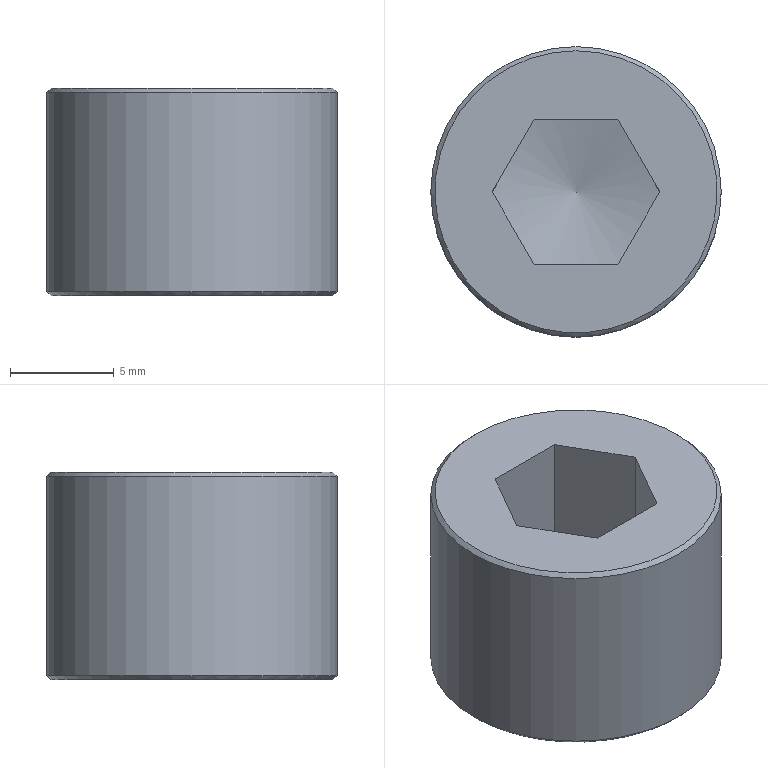Part | NX | features MFD10-WL40_3 2 | 1 solid | 18 faces | box 14 x 14 x 10 mm | volume 1223 mm3 | plane 14 | cone 3 | cylinder 1 | commonest cylinder face diameters 14 x1
STEP:
#1=CARTESIAN_POINT('',(275.029,-404.95,147.75));
#2=VERTEX_POINT('',#1);
#3=CARTESIAN_POINT('',(275.029,-411.95,147.75));
#4=DIRECTION('',(0.,0.,1.));
#5=DIRECTION('',(0.,-1.,0.));
#6=AXIS2_PLACEMENT_3D('',#3,#4,#5);
#7=CIRCLE('',#6,7.);
#8=EDGE_CURVE('',#2,#2,#7,.T.);
#9=ORIENTED_EDGE('',*,*,#8,.T.);
#10=EDGE_LOOP('',(#9));
#11=FACE_BOUND('',#10,.T.);
#12=CARTESIAN_POINT('',(275.029,-405.15,147.95));
#13=VERTEX_POINT('',#12);
#14=CARTESIAN_POINT('',(275.029,-411.95,147.95));
#15=DIRECTION('',(0.,0.,-1.));
#16=DIRECTION('',(0.,-1.,0.));
#17=AXIS2_PLACEMENT_3D('',#14,#15,#16);
#18=CIRCLE('',#17,6.8);
#19=EDGE_CURVE('',#13,#13,#18,.T.);
#20=ORIENTED_EDGE('',*,*,#19,.T.);
#21=EDGE_LOOP('',(#20));
#22=FACE_BOUND('',#21,.T.);
#23=CARTESIAN_POINT('',(275.029,-411.95,147.95));
#24=DIRECTION('',(0.,0.,-1.));
#25=DIRECTION('',(0.,-1.,0.));
#26=AXIS2_PLACEMENT_3D('',#23,#24,#25);
#27=CONICAL_SURFACE('',#26,6.8,0.7854);
#28=ADVANCED_FACE('',(#11,#22),#27,.T.);
#29=CARTESIAN_POINT('',(275.029,-404.95,138.15));
#30=VERTEX_POINT('',#29);
#31=CARTESIAN_POINT('',(275.029,-411.95,138.15));
#32=DIRECTION('',(0.,0.,-1.));
#33=DIRECTION('',(0.,-1.,0.));
#34=AXIS2_PLACEMENT_3D('',#31,#32,#33);
#35=CIRCLE('',#34,7.);
#36=EDGE_CURVE('',#30,#30,#35,.T.);
#37=ORIENTED_EDGE('',*,*,#36,.F.);
#38=EDGE_LOOP('',(#37));
#39=FACE_BOUND('',#38,.T.);
#40=ORIENTED_EDGE('',*,*,#8,.F.);
#41=EDGE_LOOP('',(#40));
#42=FACE_BOUND('',#41,.T.);
#43=CARTESIAN_POINT('',(275.029,-411.95,142.95));
#44=DIRECTION('',(0.,0.,-1.));
#45=DIRECTION('',(0.,1.,0.));
#46=AXIS2_PLACEMENT_3D('',#43,#44,#45);
#47=CYLINDRICAL_SURFACE('',#46,7.);
#48=ADVANCED_FACE('',(#39,#42),#47,.T.);
#49=CARTESIAN_POINT('',(270.987,-411.95,147.95));
#50=VERTEX_POINT('',#49);
#51=CARTESIAN_POINT('',(273.008,-408.45,147.95));
#52=VERTEX_POINT('',#51);
#53=CARTESIAN_POINT('',(271.997,-410.2,147.95));
#54=DIRECTION('',(0.5,0.866,0.));
#55=VECTOR('',#54,1000.);
#56=LINE('',#53,#55);
#57=EDGE_CURVE('',#50,#52,#56,.T.);
#58=ORIENTED_EDGE('',*,*,#57,.T.);
#59=CARTESIAN_POINT('',(277.049,-408.45,147.95));
#60=VERTEX_POINT('',#59);
#61=CARTESIAN_POINT('',(275.029,-408.45,147.95));
#62=DIRECTION('',(1.,0.,0.));
#63=VECTOR('',#62,1000.);
#64=LINE('',#61,#63);
#65=EDGE_CURVE('',#52,#60,#64,.T.);
#66=ORIENTED_EDGE('',*,*,#65,.T.);
#67=CARTESIAN_POINT('',(279.07,-411.95,147.95));
#68=VERTEX_POINT('',#67);
#69=CARTESIAN_POINT('',(278.06,-410.2,147.95));
#70=DIRECTION('',(0.5,-0.866,0.));
#71=VECTOR('',#70,1000.);
#72=LINE('',#69,#71);
#73=EDGE_CURVE('',#60,#68,#72,.T.);
#74=ORIENTED_EDGE('',*,*,#73,.T.);
#75=CARTESIAN_POINT('',(277.049,-415.45,147.95));
#76=VERTEX_POINT('',#75);
#77=CARTESIAN_POINT('',(278.06,-413.7,147.95));
#78=DIRECTION('',(-0.5,-0.866,0.));
#79=VECTOR('',#78,1000.);
#80=LINE('',#77,#79);
#81=EDGE_CURVE('',#68,#76,#80,.T.);
#82=ORIENTED_EDGE('',*,*,#81,.T.);
#83=CARTESIAN_POINT('',(273.008,-415.45,147.95));
#84=VERTEX_POINT('',#83);
#85=CARTESIAN_POINT('',(275.029,-415.45,147.95));
#86=DIRECTION('',(-1.,0.,0.));
#87=VECTOR('',#86,1000.);
#88=LINE('',#85,#87);
#89=EDGE_CURVE('',#76,#84,#88,.T.);
#90=ORIENTED_EDGE('',*,*,#89,.T.);
#91=CARTESIAN_POINT('',(271.997,-413.7,147.95));
#92=DIRECTION('',(-0.5,0.866,0.));
#93=VECTOR('',#92,1000.);
#94=LINE('',#91,#93);
#95=EDGE_CURVE('',#84,#50,#94,.T.);
#96=ORIENTED_EDGE('',*,*,#95,.T.);
#97=EDGE_LOOP('',(#58,#66,#74,#82,#90,#96));
#98=FACE_BOUND('',#97,.T.);
#99=ORIENTED_EDGE('',*,*,#19,.F.);
#100=EDGE_LOOP('',(#99));
#101=FACE_BOUND('',#100,.T.);
#102=CARTESIAN_POINT('',(275.029,-411.95,147.95));
#103=DIRECTION('',(0.,0.,1.));
#104=DIRECTION('',(0.,-1.,0.));
#105=AXIS2_PLACEMENT_3D('',#102,#103,#104);
#106=PLANE('',#105);
#107=ADVANCED_FACE('',(#98,#101),#106,.T.);
#108=ORIENTED_EDGE('',*,*,#36,.T.);
#109=EDGE_LOOP('',(#108));
#110=FACE_BOUND('',#109,.T.);
#111=CARTESIAN_POINT('',(275.029,-405.15,137.95));
#112=VERTEX_POINT('',#111);
#113=CARTESIAN_POINT('',(275.029,-411.95,137.95));
#114=DIRECTION('',(0.,0.,1.));
#115=DIRECTION('',(0.,-1.,0.));
#116=AXIS2_PLACEMENT_3D('',#113,#114,#115);
#117=CIRCLE('',#116,6.8);
#118=EDGE_CURVE('',#112,#112,#117,.T.);
#119=ORIENTED_EDGE('',*,*,#118,.T.);
#120=EDGE_LOOP('',(#119));
#121=FACE_BOUND('',#120,.T.);
#122=CARTESIAN_POINT('',(275.029,-411.95,137.95));
#123=DIRECTION('',(0.,0.,1.));
#124=DIRECTION('',(0.,-1.,0.));
#125=AXIS2_PLACEMENT_3D('',#122,#123,#124);
#126=CONICAL_SURFACE('',#125,6.8,0.7854);
#127=ADVANCED_FACE('',(#110,#121),#126,.T.);
#128=ORIENTED_EDGE('',*,*,#118,.F.);
#129=EDGE_LOOP('',(#128));
#130=FACE_BOUND('',#129,.T.);
#131=CARTESIAN_POINT('',(275.029,-411.95,137.95));
#132=DIRECTION('',(0.,0.,-1.));
#133=DIRECTION('',(0.,1.,0.));
#134=AXIS2_PLACEMENT_3D('',#131,#132,#133);
#135=PLANE('',#134);
#136=ADVANCED_FACE('',(#130),#135,.T.);
#137=CARTESIAN_POINT('',(270.987,-411.95,140.95));
#138=VERTEX_POINT('',#137);
#139=CARTESIAN_POINT('',(273.008,-408.45,140.95));
#140=VERTEX_POINT('',#139);
#141=CARTESIAN_POINT('',(271.997,-410.2,140.95));
#142=DIRECTION('',(0.5,0.866,0.));
#143=VECTOR('',#142,1000.);
#144=LINE('',#141,#143);
#145=EDGE_CURVE('',#138,#140,#144,.T.);
#146=ORIENTED_EDGE('',*,*,#145,.F.);
#147=CARTESIAN_POINT('',(275.029,-411.95,140.95));
#148=DIRECTION('',(0.,0.,1.));
#149=DIRECTION('',(0.,1.,0.));
#150=AXIS2_PLACEMENT_3D('',#147,#148,#149);
#151=CIRCLE('',#150,4.041);
#152=EDGE_CURVE('',#140,#138,#151,.T.);
#153=ORIENTED_EDGE('',*,*,#152,.F.);
#154=EDGE_LOOP('',(#146,#153));
#155=FACE_BOUND('',#154,.T.);
#156=CARTESIAN_POINT('',(275.029,-411.95,140.95));
#157=DIRECTION('',(0.,0.,1.));
#158=DIRECTION('',(0.,-1.,0.));
#159=AXIS2_PLACEMENT_3D('',#156,#157,#158);
#160=PLANE('',#159);
#161=ADVANCED_FACE('',(#155),#160,.F.);
#162=CARTESIAN_POINT('',(277.049,-408.45,140.95));
#163=VERTEX_POINT('',#162);
#164=CARTESIAN_POINT('',(275.029,-408.45,140.95));
#165=DIRECTION('',(1.,0.,0.));
#166=VECTOR('',#165,1000.);
#167=LINE('',#164,#166);
#168=EDGE_CURVE('',#140,#163,#167,.T.);
#169=ORIENTED_EDGE('',*,*,#168,.F.);
#170=CARTESIAN_POINT('',(275.029,-411.95,140.95));
#171=DIRECTION('',(0.,0.,1.));
#172=DIRECTION('',(0.,1.,0.));
#173=AXIS2_PLACEMENT_3D('',#170,#171,#172);
#174=CIRCLE('',#173,4.041);
#175=EDGE_CURVE('',#163,#140,#174,.T.);
#176=ORIENTED_EDGE('',*,*,#175,.F.);
#177=EDGE_LOOP('',(#169,#176));
#178=FACE_BOUND('',#177,.T.);
#179=CARTESIAN_POINT('',(275.029,-411.95,140.95));
#180=DIRECTION('',(0.,0.,1.));
#181=DIRECTION('',(0.,-1.,0.));
#182=AXIS2_PLACEMENT_3D('',#179,#180,#181);
#183=PLANE('',#182);
#184=ADVANCED_FACE('',(#178),#183,.F.);
#185=CARTESIAN_POINT('',(279.07,-411.95,140.95));
#186=VERTEX_POINT('',#185);
#187=CARTESIAN_POINT('',(278.06,-410.2,140.95));
#188=DIRECTION('',(0.5,-0.866,0.));
#189=VECTOR('',#188,1000.);
#190=LINE('',#187,#189);
#191=EDGE_CURVE('',#163,#186,#190,.T.);
#192=ORIENTED_EDGE('',*,*,#191,.F.);
#193=CARTESIAN_POINT('',(275.029,-411.95,140.95));
#194=DIRECTION('',(0.,0.,1.));
#195=DIRECTION('',(0.,1.,0.));
#196=AXIS2_PLACEMENT_3D('',#193,#194,#195);
#197=CIRCLE('',#196,4.041);
#198=EDGE_CURVE('',#186,#163,#197,.T.);
#199=ORIENTED_EDGE('',*,*,#198,.F.);
#200=EDGE_LOOP('',(#192,#199));
#201=FACE_BOUND('',#200,.T.);
#202=CARTESIAN_POINT('',(275.029,-411.95,140.95));
#203=DIRECTION('',(0.,0.,1.));
#204=DIRECTION('',(0.,-1.,0.));
#205=AXIS2_PLACEMENT_3D('',#202,#203,#204);
#206=PLANE('',#205);
#207=ADVANCED_FACE('',(#201),#206,.F.);
#208=CARTESIAN_POINT('',(277.049,-415.45,140.95));
#209=VERTEX_POINT('',#208);
#210=CARTESIAN_POINT('',(278.06,-413.7,140.95));
#211=DIRECTION('',(-0.5,-0.866,0.));
#212=VECTOR('',#211,1000.);
#213=LINE('',#210,#212);
#214=EDGE_CURVE('',#186,#209,#213,.T.);
#215=ORIENTED_EDGE('',*,*,#214,.F.);
#216=CARTESIAN_POINT('',(275.029,-411.95,140.95));
#217=DIRECTION('',(0.,0.,1.));
#218=DIRECTION('',(0.,1.,0.));
#219=AXIS2_PLACEMENT_3D('',#216,#217,#218);
#220=CIRCLE('',#219,4.041);
#221=EDGE_CURVE('',#209,#186,#220,.T.);
#222=ORIENTED_EDGE('',*,*,#221,.F.);
#223=EDGE_LOOP('',(#215,#222));
#224=FACE_BOUND('',#223,.T.);
#225=CARTESIAN_POINT('',(275.029,-411.95,140.95));
#226=DIRECTION('',(0.,0.,1.));
#227=DIRECTION('',(0.,-1.,0.));
#228=AXIS2_PLACEMENT_3D('',#225,#226,#227);
#229=PLANE('',#228);
#230=ADVANCED_FACE('',(#224),#229,.F.);
#231=CARTESIAN_POINT('',(273.008,-415.45,140.95));
#232=VERTEX_POINT('',#231);
#233=CARTESIAN_POINT('',(275.029,-415.45,140.95));
#234=DIRECTION('',(-1.,0.,0.));
#235=VECTOR('',#234,1000.);
#236=LINE('',#233,#235);
#237=EDGE_CURVE('',#209,#232,#236,.T.);
#238=ORIENTED_EDGE('',*,*,#237,.F.);
#239=CARTESIAN_POINT('',(275.029,-411.95,140.95));
#240=DIRECTION('',(0.,0.,1.));
#241=DIRECTION('',(0.,1.,0.));
#242=AXIS2_PLACEMENT_3D('',#239,#240,#241);
#243=CIRCLE('',#242,4.041);
#244=EDGE_CURVE('',#232,#209,#243,.T.);
#245=ORIENTED_EDGE('',*,*,#244,.F.);
#246=EDGE_LOOP('',(#238,#245));
#247=FACE_BOUND('',#246,.T.);
#248=CARTESIAN_POINT('',(275.029,-411.95,140.95));
#249=DIRECTION('',(0.,0.,1.));
#250=DIRECTION('',(0.,-1.,0.));
#251=AXIS2_PLACEMENT_3D('',#248,#249,#250);
#252=PLANE('',#251);
#253=ADVANCED_FACE('',(#247),#252,.F.);
#254=CARTESIAN_POINT('',(271.997,-413.7,140.95));
#255=DIRECTION('',(-0.5,0.866,0.));
#256=VECTOR('',#255,1000.);
#257=LINE('',#254,#256);
#258=EDGE_CURVE('',#232,#138,#257,.T.);
#259=ORIENTED_EDGE('',*,*,#258,.F.);
#260=CARTESIAN_POINT('',(275.029,-411.95,140.95));
#261=DIRECTION('',(0.,0.,1.));
#262=DIRECTION('',(0.,1.,0.));
#263=AXIS2_PLACEMENT_3D('',#260,#261,#262);
#264=CIRCLE('',#263,4.041);
#265=EDGE_CURVE('',#138,#232,#264,.T.);
#266=ORIENTED_EDGE('',*,*,#265,.F.);
#267=EDGE_LOOP('',(#259,#266));
#268=FACE_BOUND('',#267,.T.);
#269=CARTESIAN_POINT('',(275.029,-411.95,140.95));
#270=DIRECTION('',(0.,0.,1.));
#271=DIRECTION('',(0.,-1.,0.));
#272=AXIS2_PLACEMENT_3D('',#269,#270,#271);
#273=PLANE('',#272);
#274=ADVANCED_FACE('',(#268),#273,.F.);
#275=ORIENTED_EDGE('',*,*,#175,.T.);
#276=ORIENTED_EDGE('',*,*,#152,.T.);
#277=ORIENTED_EDGE('',*,*,#265,.T.);
#278=ORIENTED_EDGE('',*,*,#244,.T.);
#279=ORIENTED_EDGE('',*,*,#221,.T.);
#280=ORIENTED_EDGE('',*,*,#198,.T.);
#281=EDGE_LOOP('',(#275,#276,#277,#278,#279,#280));
#282=FACE_BOUND('',#281,.T.);
#283=CARTESIAN_POINT('',(275.029,-411.95,139.95));
#284=VERTEX_POINT('',#283);
#285=VERTEX_LOOP('',#284);
#286=FACE_BOUND('',#285,.T.);
#287=CARTESIAN_POINT('',(275.029,-411.95,140.45));
#288=DIRECTION('',(0.,0.,1.));
#289=DIRECTION('',(0.,1.,0.));
#290=AXIS2_PLACEMENT_3D('',#287,#288,#289);
#291=CONICAL_SURFACE('',#290,2.021,1.328);
#292=ADVANCED_FACE('',(#282,#286),#291,.F.);
#293=CARTESIAN_POINT('',(270.987,-411.95,144.45));
#294=DIRECTION('',(0.,0.,1.));
#295=VECTOR('',#294,1000.);
#296=LINE('',#293,#295);
#297=EDGE_CURVE('',#138,#50,#296,.T.);
#298=ORIENTED_EDGE('',*,*,#297,.F.);
#299=ORIENTED_EDGE('',*,*,#145,.T.);
#300=CARTESIAN_POINT('',(273.008,-408.45,144.45));
#301=DIRECTION('',(0.,0.,1.));
#302=VECTOR('',#301,1000.);
#303=LINE('',#300,#302);
#304=EDGE_CURVE('',#140,#52,#303,.T.);
#305=ORIENTED_EDGE('',*,*,#304,.T.);
#306=ORIENTED_EDGE('',*,*,#57,.F.);
#307=EDGE_LOOP('',(#298,#299,#305,#306));
#308=FACE_BOUND('',#307,.T.);
#309=CARTESIAN_POINT('',(271.997,-410.2,144.45));
#310=DIRECTION('',(0.866,-0.5,0.));
#311=DIRECTION('',(0.,0.,-1.));
#312=AXIS2_PLACEMENT_3D('',#309,#310,#311);
#313=PLANE('',#312);
#314=ADVANCED_FACE('',(#308),#313,.T.);
#315=CARTESIAN_POINT('',(273.008,-415.45,144.45));
#316=DIRECTION('',(0.,0.,1.));
#317=VECTOR('',#316,1000.);
#318=LINE('',#315,#317);
#319=EDGE_CURVE('',#232,#84,#318,.T.);
#320=ORIENTED_EDGE('',*,*,#319,.F.);
#321=ORIENTED_EDGE('',*,*,#258,.T.);
#322=ORIENTED_EDGE('',*,*,#297,.T.);
#323=ORIENTED_EDGE('',*,*,#95,.F.);
#324=EDGE_LOOP('',(#320,#321,#322,#323));
#325=FACE_BOUND('',#324,.T.);
#326=CARTESIAN_POINT('',(271.997,-413.7,144.45));
#327=DIRECTION('',(0.866,0.5,0.));
#328=DIRECTION('',(0.,0.,1.));
#329=AXIS2_PLACEMENT_3D('',#326,#327,#328);
#330=PLANE('',#329);
#331=ADVANCED_FACE('',(#325),#330,.T.);
#332=CARTESIAN_POINT('',(277.049,-415.45,144.45));
#333=DIRECTION('',(0.,0.,1.));
#334=VECTOR('',#333,1000.);
#335=LINE('',#332,#334);
#336=EDGE_CURVE('',#209,#76,#335,.T.);
#337=ORIENTED_EDGE('',*,*,#336,.F.);
#338=ORIENTED_EDGE('',*,*,#237,.T.);
#339=ORIENTED_EDGE('',*,*,#319,.T.);
#340=ORIENTED_EDGE('',*,*,#89,.F.);
#341=EDGE_LOOP('',(#337,#338,#339,#340));
#342=FACE_BOUND('',#341,.T.);
#343=CARTESIAN_POINT('',(275.029,-415.45,144.45));
#344=DIRECTION('',(0.,1.,0.));
#345=DIRECTION('',(0.,0.,1.));
#346=AXIS2_PLACEMENT_3D('',#343,#344,#345);
#347=PLANE('',#346);
#348=ADVANCED_FACE('',(#342),#347,.T.);
#349=CARTESIAN_POINT('',(279.07,-411.95,144.45));
#350=DIRECTION('',(0.,0.,1.));
#351=VECTOR('',#350,1000.);
#352=LINE('',#349,#351);
#353=EDGE_CURVE('',#186,#68,#352,.T.);
#354=ORIENTED_EDGE('',*,*,#353,.F.);
#355=ORIENTED_EDGE('',*,*,#214,.T.);
#356=ORIENTED_EDGE('',*,*,#336,.T.);
#357=ORIENTED_EDGE('',*,*,#81,.F.);
#358=EDGE_LOOP('',(#354,#355,#356,#357));
#359=FACE_BOUND('',#358,.T.);
#360=CARTESIAN_POINT('',(278.06,-413.7,144.45));
#361=DIRECTION('',(-0.866,0.5,0.));
#362=DIRECTION('',(0.,0.,1.));
#363=AXIS2_PLACEMENT_3D('',#360,#361,#362);
#364=PLANE('',#363);
#365=ADVANCED_FACE('',(#359),#364,.T.);
#366=CARTESIAN_POINT('',(277.049,-408.45,144.45));
#367=DIRECTION('',(0.,0.,1.));
#368=VECTOR('',#367,1000.);
#369=LINE('',#366,#368);
#370=EDGE_CURVE('',#163,#60,#369,.T.);
#371=ORIENTED_EDGE('',*,*,#370,.F.);
#372=ORIENTED_EDGE('',*,*,#191,.T.);
#373=ORIENTED_EDGE('',*,*,#353,.T.);
#374=ORIENTED_EDGE('',*,*,#73,.F.);
#375=EDGE_LOOP('',(#371,#372,#373,#374));
#376=FACE_BOUND('',#375,.T.);
#377=CARTESIAN_POINT('',(278.06,-410.2,144.45));
#378=DIRECTION('',(-0.866,-0.5,0.));
#379=DIRECTION('',(0.,0.,-1.));
#380=AXIS2_PLACEMENT_3D('',#377,#378,#379);
#381=PLANE('',#380);
#382=ADVANCED_FACE('',(#376),#381,.T.);
#383=ORIENTED_EDGE('',*,*,#304,.F.);
#384=ORIENTED_EDGE('',*,*,#168,.T.);
#385=ORIENTED_EDGE('',*,*,#370,.T.);
#386=ORIENTED_EDGE('',*,*,#65,.F.);
#387=EDGE_LOOP('',(#383,#384,#385,#386));
#388=FACE_BOUND('',#387,.T.);
#389=CARTESIAN_POINT('',(275.029,-408.45,144.45));
#390=DIRECTION('',(0.,-1.,0.));
#391=DIRECTION('',(0.,0.,-1.));
#392=AXIS2_PLACEMENT_3D('',#389,#390,#391);
#393=PLANE('',#392);
#394=ADVANCED_FACE('',(#388),#393,.T.);
#395=CLOSED_SHELL('',(#28,#48,#107,#127,#136,#161,#184,#207,#230,#253,#274,#292,#314,#331,#348,#365,#382,#394));
#396=MANIFOLD_SOLID_BREP('',#395);
#397=(LENGTH_UNIT()NAMED_UNIT(*)SI_UNIT(.MILLI.,.METRE.));
#398=UNCERTAINTY_MEASURE_WITH_UNIT(LENGTH_MEASURE(0.00001),#397,'','');
#399=(NAMED_UNIT(*)PLANE_ANGLE_UNIT()SI_UNIT($,.RADIAN.));
#400=(NAMED_UNIT(*)SI_UNIT($,.STERADIAN.)SOLID_ANGLE_UNIT());
#401=(GEOMETRIC_REPRESENTATION_CONTEXT(3)GLOBAL_UNCERTAINTY_ASSIGNED_CONTEXT((#398))GLOBAL_UNIT_ASSIGNED_CONTEXT((#397,#399,#400))REPRESENTATION_CONTEXT('',''));
#402=ADVANCED_BREP_SHAPE_REPRESENTATION('',(#396),#401);